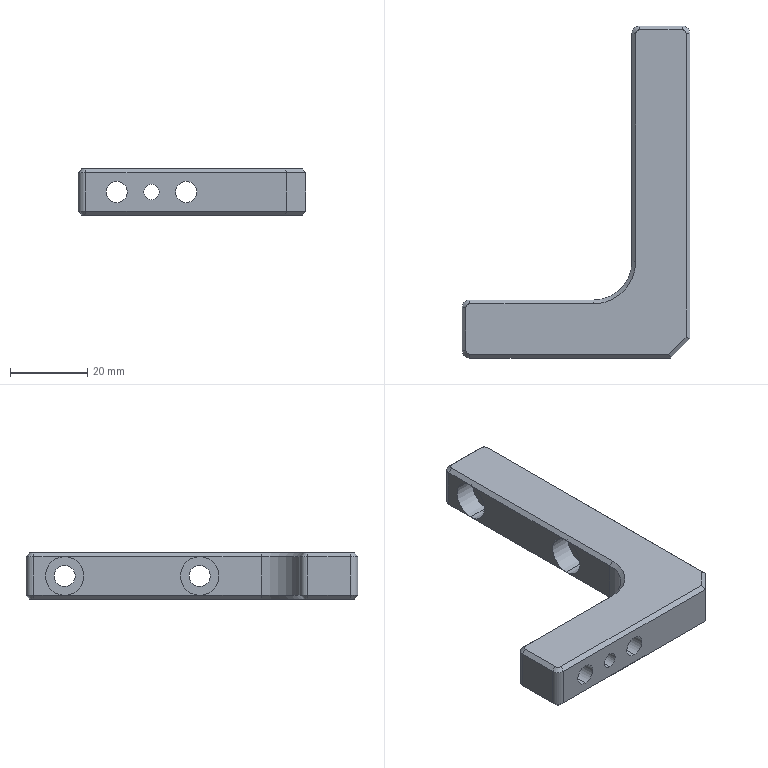Part | STEP file | 1 solid | 64 faces | box 59 x 86 x 12 mm | volume 20326 mm3 | plane 31 | cylinder 23 | cone 10 | commonest cylinder face diameters 5.5 x8 10 x8 4 x6 20 x1